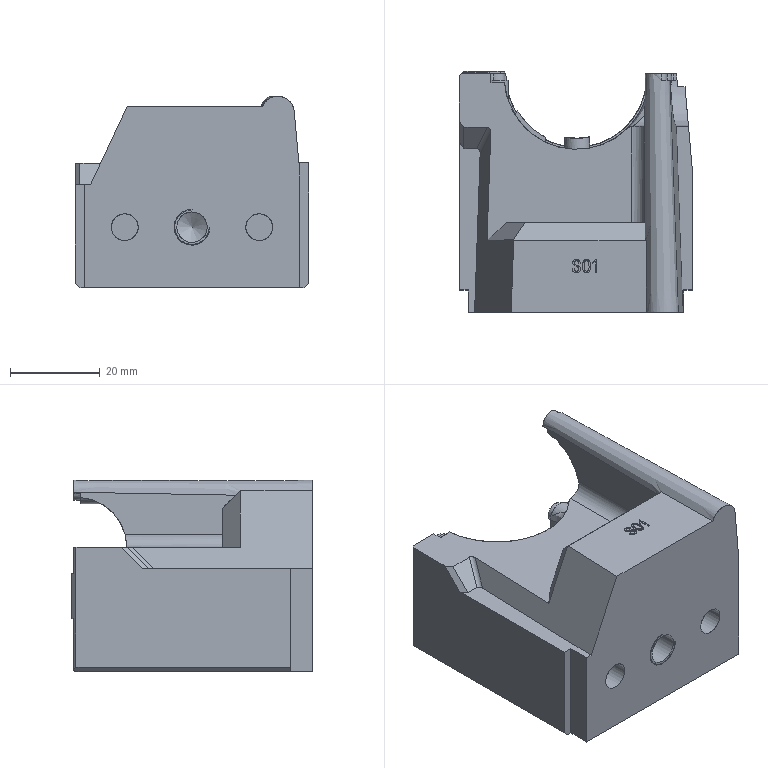NC program | PowerMill | posted with a generic post | part box 52 x 53.756 x 42.711 mm
Lines 1 to 781 of 33054:
%
O0001
N104 ( POWERMILL CB  : 2026004.0)
N105 ( POST VER      : 2026.0.0.5161)
N106 ( OPTION FILE   : FANUC)
N107 ( OUTPUT WORKPLANE : 2)
N108 (  )
N109 ( TOOL LIST )
N110 (--------------------------------------)
N111 ( NO. | ID       | DIA.| TIP RAD|LENGTH)
N112 (--------------------------------------)
N113 (    1|R3_2_1_1_1| 6.0 |  3.0   |116.4 )
N114 (--------------------------------------)
N115 (  )
N116 ( NUMBER OF TOOLPATHS: 3.0 )
N117 ( ESTIMATED PROGRAM DURATION: 0 HOURS 5 MIN 51 SEC)
N118 (  )
N119 G00 G21 G80 G40 G17
N120 G90
N121 G54
N122 G53 Z0.0
N123 (---------------)
N124 ( START TOOLPATH : 11精光-R3-平行-已选面 )
N125 (---------------)
N126 ( TOOL NO.    :1 )
N127 ( TOOL TYPE   : BALLNOSED)
N128 ( TOOL ID     : R3_2_1_1_1)
N129 ( TOOL DIA    : 6.0 LENGTH 116.4)
N130 T1
N131 M6
N132 S6500 M03
N133 G00 G90 X10.4333 Y13.1169
N134 G43 Z75.756 H1
N135
N136 G05 P10000 R8
N137 Z46.5417
N138 G01 Z43.5417 F1320.0
N139 X10.4271 Y13.1081 Z43.532 F2200.0
N140 X10.3824 Y13.0442 Z43.4586
N141 X10.3393 Y12.9826 Z43.3823
N142 X10.2207 Y12.9353 Z43.1806
N143 X10.3021 Y13.0515 Z43.3219
N144 X10.3679 Y13.1456 Z43.4349
N145 X10.4213 Y13.2218 Z43.5228
N146 X10.4589 Y13.2755 Z43.5816
N147 X10.4669 Y13.409 Z43.5938
N148 X10.4432 Y13.3752 Z43.557
N149 X10.3961 Y13.3079 Z43.4807
N150 X10.3599 Y13.2561 Z43.4208
N151 X10.3203 Y13.1995 Z43.353
N152 X10.2749 Y13.1348 Z43.277
N153 X10.2273 Y13.0668 Z43.1979
N154 X10.1799 Y12.9991 Z43.1187
N155 X10.1328 Y12.9319 Z43.0387
N156 X10.0449 Y12.9283 Z42.9006
N157 X10.1161 Y13.0301 Z43.0183
N158 X10.1883 Y13.1331 Z43.1342
N159 X10.2598 Y13.2353 Z43.2513
N160 X10.3062 Y13.3015 Z43.329
N161 X10.3447 Y13.3566 Z43.3951
N162 X10.3775 Y13.4034 Z43.4502
N163 X10.4057 Y13.4436 Z43.4981
N164 X10.4346 Y13.4849 Z43.5446
N165 X10.4688 Y13.5338 Z43.5968
N166 X10.4692 Y13.6563 Z43.5973
N167 X10.4686 Y13.6555 Z43.5964
N168 X10.4379 Y13.6117 Z43.5484
N169 X10.4077 Y13.5685 Z43.4996
N170 X10.3776 Y13.5256 Z43.4504
N171 X10.3479 Y13.4832 Z43.4006
N172 X10.3103 Y13.4295 Z43.3359
N173 X10.2651 Y13.3649 Z43.2603
N174 X10.1891 Y13.2563 Z43.1351
N175 X10.1121 Y13.1464 Z43.0116
N176 X10.0346 Y13.0356 Z42.8891
N177 X9.957 Y12.9248 Z42.7668
N178 X9.87 Y12.9227 Z42.6381
N179 X9.9413 Y13.0245 Z42.7498
N180 X10.0136 Y13.1277 Z42.8596
N181 X10.0854 Y13.2303 Z42.9703
N182 X10.1564 Y13.3317 Z43.0826
N183 X10.2253 Y13.43 Z43.1941
N184 X10.3084 Y13.5487 Z43.333
N185 X10.3456 Y13.6019 Z43.3962
N186 X10.3777 Y13.6477 Z43.4513
N187 X10.4105 Y13.6945 Z43.5052
N188 X10.4455 Y13.7445 Z43.5615
N189 X10.469 Y13.778 Z43.5975
N190 X10.4692 Y13.9004 Z43.5973
N191 X10.4419 Y13.8614 Z43.5554
N192 X10.4115 Y13.8181 Z43.5067
N193 X10.3816 Y13.7753 Z43.4572
N194 X10.3519 Y13.7329 Z43.4073
N195 X10.3159 Y13.6815 Z43.3454
N196 X10.2787 Y13.6284 Z43.283
N197 X10.2101 Y13.5304 Z43.1692
N198 X10.1452 Y13.4376 Z43.0647
N199 X10.0741 Y13.3362 Z42.9525
N200 X10.0022 Y13.2335 Z42.8419
N201 X9.9294 Y13.1295 Z42.733
N202 X9.8563 Y13.0252 Z42.6247
N203 X9.7842 Y12.9221 Z42.5146
N204 X9.6987 Z42.3953
N205 X9.7712 Y13.0256 Z42.5021
N206 X9.8441 Y13.1298 Z42.608
N207 X9.9169 Y13.2337 Z42.7141
N208 X9.989 Y13.3367 Z42.8218
N209 X10.0603 Y13.4384 Z42.931
N210 X10.1308 Y13.5392 Z43.0417
N211 X10.2285 Y13.6787 Z43.1996
N212 X10.3178 Y13.8063 Z43.3485
N213 X10.3662 Y13.8753 Z43.4313
N214 X10.4078 Y13.9348 Z43.5009
N215 X10.4597 Y14.0089 Z43.5827
N216 X10.4691 Y14.0224 Z43.5973
N217 X10.4688 Y14.144 Z43.5975
N218 X10.4383 Y14.1004 Z43.5501
N219 X10.4048 Y14.0526 Z43.4967
N220 X10.3679 Y13.9998 Z43.4343
N221 X10.3304 Y13.9463 Z43.37
N222 X10.2928 Y13.8925 Z43.3061
N223 X10.2242 Y13.7946 Z43.1925
N224 X10.1434 Y13.6792 Z43.0616
N225 X10.079 Y13.5872 Z42.9605
N226 X10.0141 Y13.4946 Z42.8603
N227 X9.9488 Y13.4013 Z42.7611
N228 X9.8827 Y13.3069 Z42.6634
N229 X9.8158 Y13.2114 Z42.5674
N230 X9.7485 Y13.1152 Z42.4722
N231 X9.6813 Y13.0193 Z42.3767
N232 X9.6145 Y12.9239 Z42.2803
N233 X9.5303 Y12.9256 Z42.1684
N234 X9.5994 Y13.0243 Z42.2655
N235 X9.6689 Y13.1237 Z42.3616
N236 X9.7386 Y13.2232 Z42.4575
N237 X9.8076 Y13.3217 Z42.5548
N238 X9.8758 Y13.4191 Z42.6537
N239 X9.9436 Y13.5159 Z42.7537
N240 X10.0107 Y13.6118 Z42.8548
N241 X10.0985 Y13.7372 Z42.9909
N242 X10.1853 Y13.861 Z43.1292
N243 X10.2709 Y13.9833 Z43.2696
N244 X10.3095 Y14.0385 Z43.3344
N245 X10.3504 Y14.0969 Z43.4047
N246 X10.3816 Y14.1415 Z43.4573
N247 X10.4089 Y14.1804 Z43.5035
N248 X10.437 Y14.2206 Z43.5481
N249 X10.4691 Y14.2664 Z43.5973
N250 Y14.3885
N251 X10.441 Y14.3483 Z43.5544
N252 X10.4118 Y14.3067 Z43.5083
N253 X10.3775 Y14.2576 Z43.4502
N254 X10.3448 Y14.211 Z43.3953
N255 X10.3073 Y14.1573 Z43.3307
N256 X10.2042 Y14.0102 Z43.16
N257 X10.1205 Y13.8906 Z43.0253
N258 X10.0356 Y13.7694 Z42.8929
N259 X9.9496 Y13.6466 Z42.7628
N260 X9.8627 Y13.5224 Z42.6346
N261 X9.7748 Y13.3969 Z42.5083
N262 X9.6859 Y13.2699 Z42.3842
N263 X9.5692 Y13.1033 Z42.2251
N264 X9.446 Y12.9273 Z42.0586
N265 X9.3616 Y12.9288 Z41.9518
N266 X9.4405 Y13.0414 Z42.0575
N267 X9.5201 Y13.1552 Z42.1614
N268 X9.5993 Y13.2683 Z42.2662
N269 X9.6778 Y13.3804 Z42.3728
N270 X9.7555 Y13.4914 Z42.481
N271 X9.8634 Y13.6455 Z42.6356
N272 X9.9675 Y13.7942 Z42.7896
N273 X10.0736 Y13.9457 Z42.9517
N274 X10.1601 Y14.0692 Z43.0884
N275 X10.2534 Y14.2025 Z43.2408
N276 X10.3154 Y14.291 Z43.3446
N277 X10.353 Y14.3447 Z43.4094
N278 X10.385 Y14.3904 Z43.4628
N279 X10.4162 Y14.435 Z43.5152
N280 X10.4418 Y14.4715 Z43.5562
N281 X10.4692 Y14.5106 Z43.5972
N282 X10.4686 Y14.6318 Z43.5977
N283 X10.4408 Y14.5921 Z43.5529
N284 X10.3672 Y14.487 Z43.4323
N285 X10.3013 Y14.3929 Z43.3208
N286 X10.2358 Y14.2993 Z43.2111
N287 X10.173 Y14.2097 Z43.1093
N288 X10.0867 Y14.0864 Z42.9722
N289 X9.9992 Y13.9614 Z42.8373
N290 X9.9106 Y13.8349 Z42.7046
N291 X9.8077 Y13.688 Z42.5552
N292 X9.7035 Y13.5392 Z42.4086
N293 X9.6438 Y13.4539 Z42.3264
N294 X9.5837 Y13.368 Z42.2451
N295 X9.5231 Y13.2815 Z42.1649
N296 X9.4621 Y13.1943 Z42.0856
N297 X9.4007 Y13.1067 Z42.0072
N298 X9.3393 Y13.019 Z41.9287
N299 X9.2787 Y12.9324 Z41.8486
N300 X9.1961 Y12.9366 Z41.7488
N301 X9.2685 Y13.04 Z41.8409
N302 X9.3413 Y13.1439 Z41.9323
N303 X9.414 Y13.2477 Z42.0238
N304 X9.4861 Y13.3507 Z42.1166
N305 X9.5576 Y13.4528 Z42.2109
N306 X9.6285 Y13.554 Z42.3066
N307 X9.706 Y13.6648 Z42.4122
N308 X9.7829 Y13.7746 Z42.5193
N309 X9.8586 Y13.8827 Z42.629
N310 X9.9339 Y13.9903 Z42.7394
N311 X10.0246 Y14.1198 Z42.8756
N312 X10.114 Y14.2474 Z43.0145
N313 X10.202 Y14.3731 Z43.156
N314 X10.2599 Y14.4559 Z43.2516
N315 X10.2969 Y14.5087 Z43.3132
N316 X10.3415 Y14.5724 Z43.3896
N317 X10.3719 Y14.6158 Z43.4409
N318 X10.399 Y14.6544 Z43.4871
N319 X10.4268 Y14.6941 Z43.5318
N320 X10.4689 Y14.7542 Z43.5974
N321 X10.4686 Y14.8759 Z43.5977
N322 X10.4304 Y14.8213 Z43.5374
N323 X10.3902 Y14.7639 Z43.4724
N324 X10.3398 Y14.692 Z43.3868
N325 X10.2844 Y14.6129 Z43.2922
N326 X10.2119 Y14.5093 Z43.1723
N327 X10.1121 Y14.3668 Z43.0122
N328 X10.0278 Y14.2464 Z42.8811
N329 X9.9426 Y14.1246 Z42.7522
N330 X9.8563 Y14.0015 Z42.6251
N331 X9.7691 Y13.8769 Z42.5002
N332 X9.6808 Y13.7508 Z42.3774
N333 X9.5687 Y13.5907 Z42.2254
N334 X9.4636 Y13.4406 Z42.0873
N335 X9.3768 Y13.3167 Z41.9764
N336 X9.2892 Y13.1916 Z41.8675
N337 X9.2011 Y13.0657 Z41.76
N338 X9.1135 Y12.9407 Z41.651
N339 X9.031 Y12.9448 Z41.5548
N340 X9.1135 Y13.0626 Z41.6557
N341 X9.1967 Y13.1815 Z41.7546
N342 X9.2794 Y13.2996 Z41.8551
N343 X9.3613 Y13.4166 Z41.9574
N344 X9.4427 Y13.5329 Z42.0609
N345 X9.5469 Y13.6816 Z42.1966
N346 X9.6499 Y13.8287 Z42.3349
N347 X9.7442 Y13.9634 Z42.4651
N348 X9.8374 Y14.0965 Z42.5979
N349 X9.9296 Y14.2281 Z42.7328
N350 X10.0207 Y14.3582 Z42.8699
N351 X10.1105 Y14.4865 Z43.0095
N352 X10.2086 Y14.6267 Z43.1671
N353 X10.3083 Y14.7691 Z43.3326
N354 X10.3471 Y14.8245 Z43.3992
N355 X10.3794 Y14.8706 Z43.4536
N356 X10.4179 Y14.9255 Z43.518
N357 X10.4447 Y14.9638 Z43.5605
N358 X10.4692 Y14.9988 Z43.5972
N359 X10.4691 Y15.1208 Z43.5973
N360 X10.4664 Y15.1168 Z43.5931
N361 X10.4195 Y15.0499 Z43.5205
N362 X10.3801 Y14.9936 Z43.4551
N363 X10.3366 Y14.9315 Z43.3806
N364 X10.2421 Y14.7965 Z43.2219
N365 X10.1486 Y14.663 Z43.0699
N366 X10.055 Y14.5293 Z42.9229
N367 X9.958 Y14.3908 Z42.7752
N368 X9.8597 Y14.2503 Z42.6302
N369 X9.76 Y14.108 Z42.4879
N370 X9.6453 Y13.9442 Z42.3288
N371 X9.5338 Y13.785 Z42.1791
N372 X9.425 Y13.6296 Z42.0376
N373 X9.3466 Y13.5176 Z41.9387
N374 X9.2678 Y13.405 Z41.8409
N375 X9.1884 Y13.2917 Z41.7444
N376 X9.1083 Y13.1772 Z41.6499
N377 X9.0279 Y13.0624 Z41.5559
N378 X8.9479 Y12.9482 Z41.4609
N379 X8.8631 Y12.9491 Z41.3656
N380 X9.0072 Y13.155 Z41.5314
N381 X9.073 Y13.249 Z41.6077
N382 X9.13 Y13.3303 Z41.675
N383 X9.1867 Y13.4113 Z41.7429
N384 X9.2433 Y13.4921 Z41.8113
N385 X9.2997 Y13.5726 Z41.8801
N386 X9.3558 Y13.6527 Z41.9496
N387 X9.4114 Y13.7321 Z42.0203
N388 X9.5162 Y13.8818 Z42.1559
N389 X9.6198 Y14.0298 Z42.2942
N390 X9.7223 Y14.1762 Z42.435
N391 X9.8237 Y14.3211 Z42.5782
N392 X9.925 Y14.4658 Z42.726
N393 X10.025 Y14.6084 Z42.8767
N394 X10.1235 Y14.7492 Z43.0301
N395 X10.2041 Y14.8643 Z43.1596
N396 X10.2989 Y14.9997 Z43.3167
N397 X10.3348 Y15.0509 Z43.3778
N398 X10.3664 Y15.0961 Z43.4318
N399 X10.3983 Y15.1416 Z43.4854
N400 X10.4275 Y15.1833 Z43.5336
N401 X10.4595 Y15.2291 Z43.5827
N402 X10.4691 Y15.2428 Z43.5972
N403 Y15.3648 Z43.5973
N404 X10.4579 Y15.3488 Z43.5799
N405 X10.4066 Y15.2755 Z43.4989
N406 X10.3657 Y15.2171 Z43.4305
N407 X10.3223 Y15.1551 Z43.3561
N408 X10.2471 Y15.0477 Z43.2302
N409 X10.1545 Y14.9154 Z43.0794
N410 X10.0574 Y14.7769 Z42.9265
N411 X9.9788 Y14.6645 Z42.8064
N412 X9.8992 Y14.5509 Z42.6881
N413 X9.8189 Y14.4363 Z42.5713
N414 X9.7378 Y14.3204 Z42.4563
N415 X9.6558 Y14.2033 Z42.3432
N416 X9.5629 Y14.0706 Z42.2175
N417 X9.469 Y13.9365 Z42.0942
N418 X9.374 Y13.8008 Z41.9734
N419 X9.3009 Y13.6964 Z41.8824
N420 X9.2275 Y13.5915 Z41.7921
N421 X9.1536 Y13.4861 Z41.7029
N422 X9.0793 Y13.3799 Z41.6151
N423 X9.0043 Y13.2728 Z41.5289
N424 X8.9288 Y13.1651 Z41.4437
N425 X8.8534 Y13.0573 Z41.3586
N426 X8.7781 Y12.9498 Z41.2731
N427 X8.69 Y12.946 Z41.1786
N428 X8.7517 Y13.0341 Z41.2465
N429 X8.8134 Y13.1223 Z41.3144
N430 X8.8751 Y13.2103 Z41.3825
N431 X8.9366 Y13.2982 Z41.451
N432 X8.9977 Y13.3855 Z41.5206
N433 X9.1329 Y13.5786 Z41.6786
N434 X9.2597 Y13.7596 Z41.8312
N435 X9.3794 Y13.9305 Z41.9798
N436 X9.4865 Y14.0835 Z42.1171
N437 X9.5924 Y14.2348 Z42.2572
N438 X9.7014 Y14.3905 Z42.4057
N439 X9.8049 Y14.5383 Z42.5512
N440 X9.9072 Y14.6843 Z42.6994
N441 X10.0062 Y14.8258 Z42.848
N442 X10.1078 Y14.9708 Z43.0055
N443 X10.2127 Y15.1206 Z43.1734
N444 X10.2753 Y15.21 Z43.2769
N445 X10.3347 Y15.2949 Z43.3775
N446 X10.376 Y15.3538 Z43.4484
N447 X10.41 Y15.4025 Z43.5046
N448 X10.4645 Y15.4802 Z43.5908
N449 X10.4687 Y15.4862 Z43.5976
N450 X10.4685 Y15.6081 Z43.5974
N451 X10.4154 Y15.5321 Z43.5119
N452 X10.3542 Y15.4448 Z43.4108
N453 X10.2962 Y15.3619 Z43.312
N454 X10.2276 Y15.264 Z43.1979
N455 X10.1551 Y15.1605 Z43.0807
N456 X10.0582 Y15.0221 Z42.9278
N457 X9.967 Y14.8918 Z42.7886
N458 X9.8716 Y14.7555 Z42.6473
N459 X9.7749 Y14.6174 Z42.5085
N460 X9.677 Y14.4777 Z42.3722
N461 X9.587 Y14.3492 Z42.2497
N462 X9.4961 Y14.2192 Z42.1295
N463 X9.4042 Y14.088 Z42.0114
N464 X9.3116 Y13.9558 Z41.895
N465 X9.1954 Y13.7899 Z41.753
N466 X9.0724 Y13.6142 Z41.6074
N467 X8.9793 Y13.4812 Z41.5001
N468 X8.8856 Y13.3474 Z41.3947
N469 X8.7911 Y13.2124 Z41.2914
N470 X8.6961 Y13.0768 Z41.1893
N471 X8.6017 Y12.9419 Z41.0858
N472 X8.5133 Y12.9377 Z40.9946
N473 X8.6021 Y13.0646 Z41.0907
N474 X8.6917 Y13.1925 Z41.1847
N475 X8.7809 Y13.3199 Z41.2799
N476 X8.8694 Y13.4463 Z41.3768
N477 X8.9574 Y13.572 Z41.4753
N478 X9.058 Y13.7156 Z41.5907
N479 X9.1579 Y13.8583 Z41.708
N480 X9.2569 Y13.9998 Z41.8273
N481 X9.355 Y14.1398 Z41.949
N482 X9.4682 Y14.3015 Z42.0936
N483 X9.5845 Y14.4675 Z42.2468
N484 X9.6975 Y14.6289 Z42.4006
N485 X9.8049 Y14.7823 Z42.5514
N486 X9.9109 Y14.9337 Z42.7052
N487 X10.006 Y15.0696 Z42.8474
N488 X10.0864 Y15.1844 Z42.9717
N489 X10.1498 Y15.2749 Z43.0722
N490 X10.2128 Y15.3649 Z43.1735
N491 X10.2729 Y15.4507 Z43.2739
N492 X10.3328 Y15.5363 Z43.3746
N493 X10.3622 Y15.5783 Z43.4244
N494 X10.3908 Y15.6191 Z43.4734
N495 X10.4203 Y15.6612 Z43.5208
N496 X10.4564 Y15.7128 Z43.5779
N497 X10.4684 Y15.7299 Z43.5973
N498 X10.4686 Y15.8522 Z43.597
N499 X10.4682 Y15.8517 Z43.5965
N500 X10.4084 Y15.7663 Z43.5016
N501 X10.3634 Y15.702 Z43.4274
N502 X10.3003 Y15.6118 Z43.3193
N503 X10.2494 Y15.5392 Z43.2341
N504 X10.1572 Y15.4076 Z43.0842
N505 X10.0637 Y15.274 Z42.9366
N506 X9.969 Y15.1387 Z42.7916
N507 X9.8662 Y14.9919 Z42.6394
N508 X9.7596 Y14.8396 Z42.4868
N509 X9.6489 Y14.6816 Z42.3336
N510 X9.5348 Y14.5186 Z42.1804
N511 X9.419 Y14.3532 Z42.03
N512 X9.3003 Y14.1838 Z41.8809
N513 X9.1788 Y14.0102 Z41.733
N514 X9.0543 Y13.8324 Z41.5864
N515 X8.9267 Y13.6502 Z41.4409
N516 X8.844 Y13.5321 Z41.349
N517 X8.761 Y13.4135 Z41.2583
N518 X8.6773 Y13.294 Z41.1692
N519 X8.5932 Y13.1738 Z41.0815
N520 X8.5089 Y13.0535 Z40.9941
N521 X8.4249 Y12.9335 Z40.906
N522 X8.3375 Y12.9308 Z40.8191
N523 X8.496 Y13.1571 Z40.9817
N524 X8.6042 Y13.3116 Z41.0924
N525 X8.692 Y13.437 Z41.1847
N526 X8.7866 Y13.5721 Z41.2865
N527 X8.8756 Y13.6992 Z41.3836
N528 X8.9638 Y13.8252 Z41.4827
N529 X9.0515 Y13.9504 Z41.5832
N530 X9.1386 Y14.0749 Z41.6851
N531 X9.2252 Y14.1984 Z41.7887
N532 X9.3448 Y14.3693 Z41.9362
N533 X9.464 Y14.5395 Z42.0881
N534 X9.573 Y14.6952 Z42.2313
N535 X9.6808 Y14.8491 Z42.3773
N536 X9.7872 Y15.0012 Z42.5261
N537 X9.8924 Y15.1513 Z42.6778
N538 X9.9961 Y15.2994 Z42.8325
N539 X10.0854 Y15.4271 Z42.9703
N540 X10.1736 Y15.553 Z43.1104
N541 X10.2606 Y15.6773 Z43.2526
N542 X10.2991 Y15.7322 Z43.3167
N543 X10.3373 Y15.7868 Z43.3823
N544 X10.3698 Y15.8331 Z43.4371
N545 X10.3981 Y15.8736 Z43.4856
N546 X10.4273 Y15.9153 Z43.5327
N547 X10.457 Y15.9577 Z43.5787
N548 X10.4371 Y16.0514 Z43.5477
N549 X10.3596 Y15.9406 Z43.4192
N550 X10.3049 Y15.8625 Z43.327
N551 X10.2501 Y15.7843 Z43.2349
N552 X10.1947 Y15.7051 Z43.1441
N553 X10.0972 Y15.5659 Z42.9887
N554 X9.9983 Y15.4247 Z42.836
N555 X9.898 Y15.2815 Z42.686
N556 X9.7964 Y15.1363 Z42.539
N557 X9.6935 Y14.9893 Z42.3946
N558 X9.5848 Y14.8342 Z42.247
N559 X9.4749 Y14.6772 Z42.1023
N560 X9.3646 Y14.5196 Z41.9612
N561 X9.253 Y14.3603 Z41.8229
N562 X9.1404 Y14.1995 Z41.6873
N563 X9.0267 Y14.0371 Z41.5544
N564 X8.912 Y13.8733 Z41.4244
N565 X8.8306 Y13.757 Z41.3346
N566 X8.7489 Y13.6403 Z41.2458
N567 X8.6668 Y13.5231 Z41.158
N568 X8.5842 Y13.4052 Z41.0717
N569 X8.501 Y13.2863 Z40.9872
N570 X8.4175 Y13.167 Z40.9036
N571 X8.334 Y13.0478 Z40.82
N572 X8.2507 Y12.9288 Z40.7358
N573 X8.1639 Y12.9269 Z40.6529
N574 X8.2409 Y13.0369 Z40.7302
N575 X8.3184 Y13.1475 Z40.8064
N576 X8.3996 Y13.2635 Z40.8855
N577 X8.4803 Y13.3788 Z40.9663
N578 X8.6417 Y13.6093 Z41.1317
N579 X8.6887 Y13.6764 Z41.1808
N580 X8.7353 Y13.743 Z41.2309
N581 X8.7819 Y13.8094 Z41.2814
N582 X8.8283 Y13.8758 Z41.332
N583 X8.8747 Y13.942 Z41.3829
N584 X8.9209 Y14.0081 Z41.434
N585 X8.967 Y14.0739 Z41.4857
N586 X9.0128 Y14.1392 Z41.5383
N587 X9.1178 Y14.2893 Z41.6607
N588 X9.2221 Y14.4382 Z41.7852
N589 X9.3254 Y14.5857 Z41.9121
N590 X9.4341 Y14.7409 Z42.0494
N591 X9.5416 Y14.8945 Z42.1894
N592 X9.6479 Y15.0463 Z42.3322
N593 X9.7591 Y15.2051 Z42.4864
N594 X9.8684 Y15.3612 Z42.643
N595 X9.9757 Y15.5145 Z42.802
N596 X10.0811 Y15.665 Z42.9633
N597 X10.1552 Y15.7708 Z43.0799
N598 X10.2202 Y15.8636 Z43.1854
N599 X10.2844 Y15.9552 Z43.2926
N600 X10.3481 Y16.0463 Z43.4005
N601 X10.3996 Y16.1198 Z43.4865
N602 X10.3487 Y16.1691 Z43.3994
N603 X10.2783 Y16.0687 Z43.282
N604 X10.1924 Y15.946 Z43.141
N605 X10.1055 Y15.8219 Z43.0018
N606 X10.0175 Y15.6961 Z42.865
N607 X9.9282 Y15.5686 Z42.7305
N608 X9.8378 Y15.4395 Z42.5985
N609 X9.7463 Y15.3089 Z42.4685
N610 X9.654 Y15.1771 Z42.3404
N611 X9.5583 Y15.0404 Z42.2114
N612 X9.4615 Y14.9021 Z42.0848
N613 X9.3638 Y14.7626 Z41.9603
N614 X9.2653 Y14.622 Z41.8377
N615 X9.1621 Y14.4745 Z41.7131
N616 X9.0579 Y14.3258 Z41.5908
N617 X8.953 Y14.1759 Z41.4705
N618 X8.8473 Y14.0249 Z41.3522
N619 X8.7821 Y13.9318 Z41.281
N620 X8.7165 Y13.8381 Z41.2109
N621 X8.6506 Y13.7441 Z41.1414
N622 X8.5846 Y13.6498 Z41.0725
N623 X8.5184 Y13.5552 Z41.0042
N624 X8.4517 Y13.46 Z40.9371
N625 X8.3722 Y13.3464 Z40.8586
N626 X8.2662 Y13.1951 Z40.7555
N627 X8.186 Y13.0806 Z40.6789
N628 X8.0772 Y12.9251 Z40.5725
N629 X7.9908 Y12.9237 Z40.4939
N630 X8.0571 Y13.0185 Z40.5581
N631 X8.1223 Y13.1116 Z40.6201
N632 X8.1955 Y13.2162 Z40.6882
N633 X8.2683 Y13.3201 Z40.7576
N634 X8.3982 Y13.5055 Z40.8839
N635 X8.5191 Y13.6782 Z41.0051
N636 X8.639 Y13.8495 Z41.129
N637 X8.7581 Y14.0196 Z41.2555
N638 X8.8763 Y14.1884 Z41.3845
N639 X8.9935 Y14.3558 Z41.5162
N640 X9.1096 Y14.5216 Z41.6509
N641 X9.2255 Y14.6871 Z41.7894
N642 X9.3403 Y14.851 Z41.9306
N643 X9.4555 Y15.0156 Z42.077
N644 X9.5678 Y15.1759 Z42.2243
N645 X9.6787 Y15.3343 Z42.3745
N646 X9.7781 Y15.4763 Z42.5133
N647 X9.8835 Y15.6268 Z42.6647
N648 X9.9823 Y15.768 Z42.8116
N649 X10.0531 Y15.8691 Z42.9199
N650 X10.1232 Y15.9692 Z43.0296
N651 X10.1924 Y16.068 Z43.1411
N652 X10.2617 Y16.1669 Z43.2524
N653 X10.2983 Y16.2193 Z43.31
N654 X10.22 Y16.2295 Z43.1798
N655 X10.1612 Y16.1455 Z43.0896
N656 X10.0969 Y16.0536 Z42.9887
N657 X10.0238 Y15.9493 Z42.875
N658 X9.943 Y15.8339 Z42.7529
N659 X9.8369 Y15.6823 Z42.597
N660 X9.7312 Y15.5314 Z42.4469
N661 X9.6246 Y15.3791 Z42.3004
N662 X9.5096 Y15.2149 Z42.1473
N663 X9.392 Y15.047 Z41.9958
N664 X9.2718 Y14.8753 Z41.8458
N665 X9.1489 Y14.6998 Z41.6974
N666 X9.0233 Y14.5204 Z41.5506
N667 X8.895 Y14.3371 Z41.4053
N668 X8.7669 Y14.1542 Z41.2649
N669 X8.6316 Y13.961 Z41.1212
N670 X8.5113 Y13.7891 Z40.9971
N671 X8.39 Y13.6159 Z40.8759
N672 X8.2679 Y13.4415 Z40.7571
N673 X8.1735 Y13.3067 Z40.6672
N674 X8.0589 Y13.143 Z40.5609
N675 X7.9052 Y12.9236 Z40.4173
N676 X7.8196 Y12.9234 Z40.343
N677 X7.9178 Y13.0636 Z40.4338
N678 X8.0165 Y13.2045 Z40.523
N679 X8.115 Y13.3452 Z40.6126
N680 X8.2129 Y13.485 Z40.7043
N681 X8.3102 Y13.624 Z40.7977
N682 X8.4071 Y13.7624 Z40.8927
N683 X8.5285 Y13.9358 Z41.0147
N684 X8.6504 Y14.1099 Z41.1408
N685 X8.781 Y14.2964 Z41.2803
N686 X8.91 Y14.4806 Z41.4221
N687 X9.0366 Y14.6615 Z41.5659
N688 X9.1609 Y14.839 Z41.7116
N689 X9.2829 Y15.0132 Z41.8595
N690 X9.4026 Y15.1842 Z42.0093
N691 X9.5072 Y15.3335 Z42.1443
N692 X9.6107 Y15.4813 Z42.2816
N693 X9.713 Y15.6274 Z42.4216
N694 X9.7845 Y15.7295 Z42.5222
N695 X9.8554 Y15.8308 Z42.6237
N696 X9.9257 Y15.9311 Z42.7268
N697 X9.9951 Y16.0303 Z42.8315
N698 X10.0643 Y16.1291 Z42.9368
N699 X10.1341 Y16.2288 Z43.0409
N700 X10.1369 Y16.2328 Z43.0451
N701 X10.0538 Y16.2362 Z42.9144
N702 X10.0472 Y16.2267 Z42.905
N703 X9.969 Y16.1151 Z42.7918
N704 X9.8916 Y16.0046 Z42.6768
N705 X9.8135 Y15.893 Z42.5633
N706 X9.7345 Y15.7802 Z42.4518
N707 X9.6549 Y15.6665 Z42.3416
N708 X9.547 Y15.5124 Z42.1964
N709 X9.4339 Y15.3509 Z42.049
N710 X9.3151 Y15.1812 Z41.8991
N711 X9.1945 Y15.0089 Z41.7517
N712 X9.0703 Y14.8316 Z41.605
N713 X8.9425 Y14.649 Z41.4586
N714 X8.8108 Y14.4609 Z41.3125
N715 X8.6774 Y14.2705 Z41.1693
N716 X8.5412 Y14.076 Z41.0278
N717 X8.4022 Y13.8775 Z40.8879
N718 X8.2603 Y13.6748 Z40.7497
N719 X8.1154 Y13.4678 Z40.6131
N720 X8.0054 Y13.3108 Z40.5127
N721 X7.895 Y13.1531 Z40.414
N722 X7.7365 Y12.9267 Z40.2711
N723 X7.6532 Y12.9298 Z40.2015
N724 X7.7587 Y13.0805 Z40.2956
N725 X7.8648 Y13.232 Z40.3876
N726 X7.9705 Y13.383 Z40.4811
N727 X8.0756 Y13.533 Z40.5766
N728 X8.2176 Y13.7359 Z40.709
N729 X8.351 Y13.9263 Z40.8374
N730 X8.4892 Y14.1238 Z40.9749
N731 X8.6272 Y14.3208 Z41.1166
N732 X8.7632 Y14.515 Z41.2609
N733 X8.89 Y14.6962 Z41.3998
N734 X9.016 Y14.876 Z41.5421
N735 X9.1421 Y15.0561 Z41.6894
N736 X9.2572 Y15.2206 Z41.8281
N737 X9.3749 Y15.3887 Z41.9741
N738 X9.487 Y15.5487 Z42.1178
N739 X9.5585 Y15.6508 Z42.212
N740 X9.6295 Y15.7523 Z42.3071
N741 X9.7 Y15.853 Z42.4034
N742 X9.7698 Y15.9526 Z42.5014
N743 X9.839 Y16.0514 Z42.6006
N744 X9.9083 Y16.1504 Z42.6995
N745 X9.9707 Y16.2395 Z42.7873
N746 X9.887 Y16.2421 Z42.6633
N747 X9.7423 Y16.0354 Z42.4624
N748 X9.6637 Y15.9231 Z42.3533
N749 X9.5843 Y15.8097 Z42.2461
N750 X9.5042 Y15.6953 Z42.1404
N751 X9.4235 Y15.5801 Z42.0361
N752 X9.3423 Y15.4641 Z41.9331
N753 X9.2604 Y15.3471 Z41.8317
N754 X9.1382 Y15.1726 Z41.6847
N755 X9.0147 Y14.9963 Z41.5407
N756 X8.8901 Y14.8183 Z41.3999
N757 X8.7643 Y14.6387 Z41.2622
N758 X8.6375 Y14.4576 Z41.1276
N759 X8.5199 Y14.2896 Z41.0062
N760 X8.4015 Y14.1206 Z40.8871
N761 X8.2822 Y13.9501 Z40.7709
N762 X8.1706 Y13.7907 Z40.6648
N763 X8.0584 Y13.6305 Z40.5604
N764 X7.9455 Y13.4692 Z40.4585
N765 X7.8516 Y13.3351 Z40.3755
N766 X7.7223 Y13.1505 Z40.2643
N767 X7.5699 Y12.9329 Z40.1322
N768 X7.4866 Y12.9359 Z40.0651
N769 X7.5822 Y13.0725 Z40.1468
N770 X7.6781 Y13.2095 Z40.2276
N771 X7.774 Y13.3463 Z40.3085
N772 X7.8693 Y13.4825 Z40.3912
N773 X7.9642 Y13.618 Z40.4756
N774 X8.0587 Y13.753 Z40.5611
N775 X8.1986 Y13.9527 Z40.6909
N776 X8.3386 Y14.1527 Z40.8253
N777 X8.4788 Y14.353 Z40.9644
N778 X8.6074 Y14.5367 Z41.096
N779 X8.7351 Y14.7189 Z41.2305
N780 X8.8616 Y14.8996 Z41.3682
N781 X8.987 Y15.0787 Z41.509
N782 X9.1002 Y15.2404 Z41.6401
N783 X9.2229 Y15.4156 Z41.7862
N784 X9.3376 Y15.5794 Z41.9271
N785 X9.4227 Y15.701 Z42.0349
N786 X9.5072 Y15.8217 Z42.1441
N787 X9.591 Y15.9413 Z42.255
N788 X9.6739 Y16.0597 Z42.368
N789 X9.7569 Y16.1782 Z42.4807
N790 X9.802 Y16.2427 Z42.5402
N791 X9.7169 Y16.2432 Z42.4205
N792 X9.6565 Y16.1569 Z42.3415
N793 X9.5855 Y16.0555 Z42.2481
N794 X9.5146 Y15.9543 Z42.1543
N795 X9.4435 Y15.8528 Z42.0612
N796 X9.3718 Y15.7503 Z41.9697
N797 X9.2993 Y15.6468 Z41.8799
N798 X9.2264 Y15.5427 Z41.7912
N799 X9.1532 Y15.4381 Z41.7032
N800 X9.0436 Y15.2816 Z41.5742
N801 X8.9244 Y15.1114 Z41.4381
N802 X8.7974 Y14.9301 Z41.2978
N803 X8.6655 Y14.7416 Z41.1566
N804 X8.5378 Y14.5592 Z41.0241
N805 X8.4134 Y14.3816 Z40.8989
N806 X8.2727 Y14.1806 Z40.7616
N807 X8.1285 Y13.9747 Z40.6253
N808 X7.9857 Y13.7708 Z40.4947
N809 X7.8894 Y13.6333 Z40.409
N810 X7.7928 Y13.4953 Z40.3246
N811 X7.6957 Y13.3566 Z40.2418
N812 X7.5981 Y13.2172 Z40.1608
N813 X7.5004 Y13.0778 Z40.08
N814 X7.4031 Y12.9387 Z39.9981
N815 X7.3194 Y12.9412 Z39.9326
N816 X7.4355 Y13.107 Z40.0282
N817 X7.5517 Y13.2731 Z40.1231
N818 X7.6678 Y13.4388 Z40.2189
N819 X7.7832 Y13.6036 Z40.3168
N820 X7.898 Y13.7676 Z40.4169
N821 X8.0479 Y13.9816 Z40.5512
N822 X8.1913 Y14.1864 Z40.684
N823 X8.329 Y14.383 Z40.8159
N824 X8.4641 Y14.5761 Z40.9496
N825 X8.6021 Y14.7731 Z41.0905
N826 X8.7353 Y14.9634 Z41.231
N827 X8.854 Y15.1329 Z41.3601
N828 X8.9718 Y15.3011 Z41.4916
N829 X9.0885 Y15.4678 Z41.626
N830 X9.2041 Y15.6329 Z41.7633
N831 X9.3091 Y15.7829 Z41.8919
N832 X9.4229 Y15.9453 Z42.0354
N833 X9.5787 Y16.1679 Z42.2352
N834 X9.6302 Y16.2414 Z42.3012
N835 X9.5435 Y16.2396 Z42.1857
N836 X9.5369 Y16.2302 Z42.1776
N837 X9.4571 Y16.1162 Z42.0785
N838 X9.3778 Y16.003 Z41.9782
N839 X9.2983 Y15.8895 Z41.8784
N840 X9.2182 Y15.775 Z41.7802
N841 X9.1374 Y15.6596 Z41.6837
N842 X9.0561 Y15.5435 Z41.5886
N843 X8.9743 Y15.4267 Z41.4946
N844 X8.8645 Y15.27 Z41.3715
N845 X8.7539 Y15.112 Z41.2508
N846 X8.6425 Y14.9528 Z41.1326
N847 X8.5263 Y14.7869 Z41.0124
N848 X8.4092 Y14.6197 Z40.8948
N849 X8.2718 Y14.4234 Z40.7609
N850 X8.1334 Y14.2257 Z40.6299
N851 X7.994 Y14.0267 Z40.502
N852 X7.8537 Y13.8264 Z40.3772
N853 X7.7517 Y13.6806 Z40.289
N854 X7.6491 Y13.5342 Z40.2025
N855 X7.546 Y13.387 Z40.1179
N856 X7.4426 Y13.2392 Z40.0346
N857 X7.339 Y13.0913 Z39.9517
N858 X7.2356 Y12.9436 Z39.8683
N859 X7.1518 Y12.9459 Z39.8048
N860 X7.2784 Y13.1267 Z39.9052
N861 X7.4053 Y13.308 Z40.0045
N862 X7.5318 Y13.4886 Z40.1054
N863 X7.6517 Y13.6598 Z40.2045
N864 X7.7709 Y13.8301 Z40.306
N865 X7.8896 Y13.9997 Z40.4093
N866 X8.0078 Y14.1685 Z40.5146
N867 X8.1253 Y14.3362 Z40.6221
N868 X8.242 Y14.5029 Z40.7322
N869 X8.3708 Y14.6869 Z40.8568
N870 X8.4987 Y14.8696 Z40.9843
N871 X8.6275 Y15.0535 Z41.1166
N872 X8.7533 Y15.2332 Z41.2502
N873 X8.8781 Y15.4113 Z41.3869
N874 X8.9594 Y15.5275 Z41.4784
N875 X9.0367 Y15.6379 Z41.5666
N876 X9.1136 Y15.7478 Z41.6557
N877 X9.19 Y15.8569 Z41.7462
N878 X9.2657 Y15.965 Z41.8386